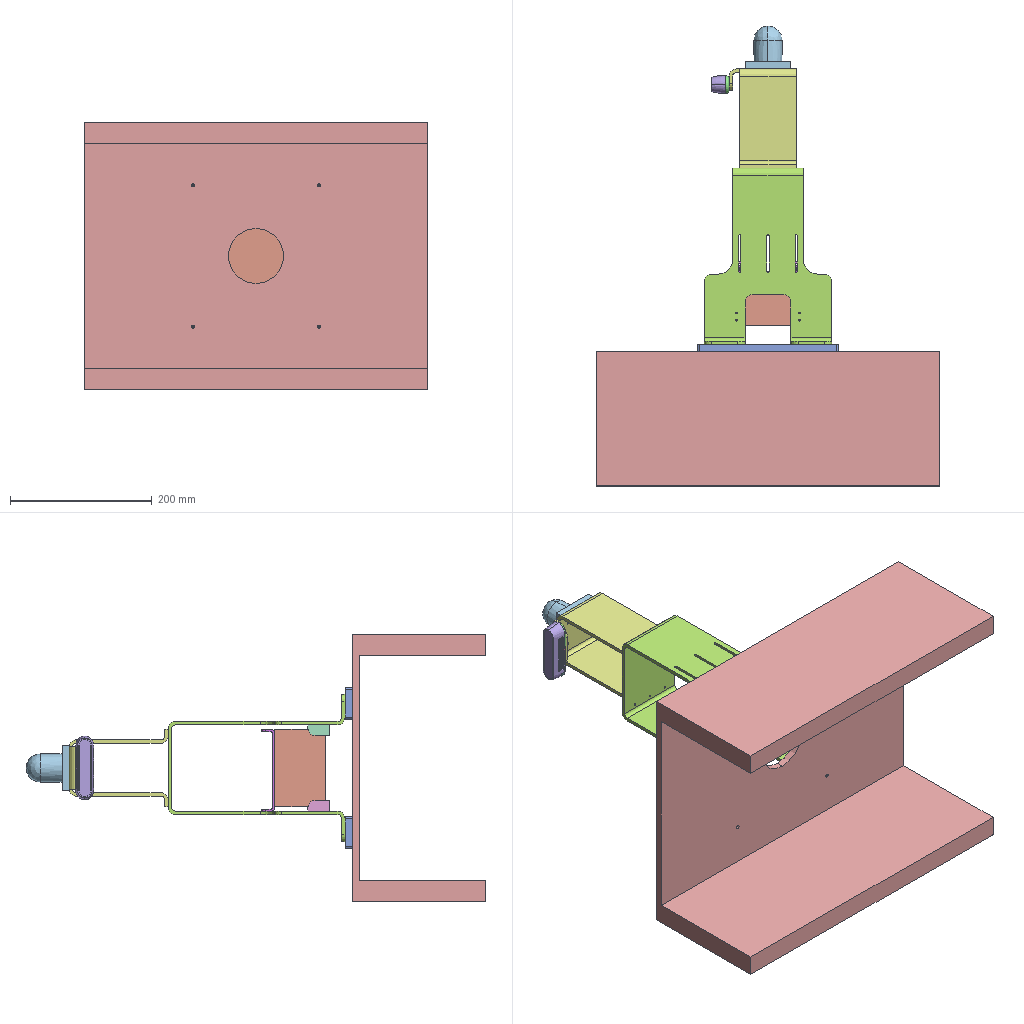Assembly | SolidWorks | 10 different items | 14 placed | box 484 x 650 x 378 mm
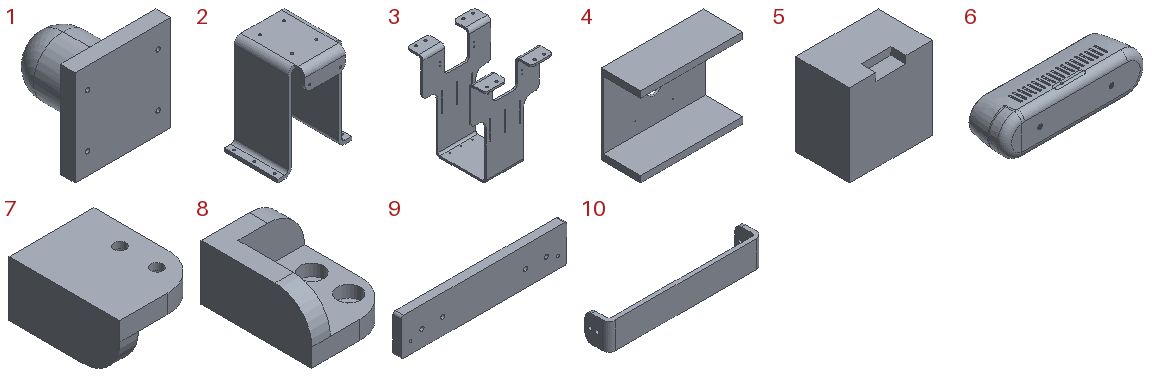Parts list (item | quantity | size | volume | features):
1 | x1 | 65 x 60.8 x 65 mm | 97568 mm3 | features ICE 2, Extrusion 1, Fillet 1
2 | x1 | 110 x 95 x 140 mm | 157187 mm3 | features ICE 7, Fillet 5, Extrusion 1
3 | x1 | 180 x 208 x 250 mm | 376013 mm3 | features ICE 8, Fillet 5, HoleWzd 2, MoveFace 2, Extrusion 1
4 | x1 | 484 x 189 x 378 mm | 6979121 mm3 | features ICE 2, Extrusion 1
5 | x1 | 110 x 72 x 110 mm | 863200 mm3 | features Extrusion 1, ICE 1
6 | x1 | 90 x 25 x 25 mm | 48696 mm3 | features ICE 13, SweepThread 3, Fillet 2, Split 2, Blend 1
7 | x2 | 23 x 30 x 15 mm | 5306 mm3 | features ICE 3, MoveFace 2, Extrusion 1, Fillet 1
8 | x2 | 23 x 30 x 15 mm | 5306 mm3 | features MirrorStock 1
9 | x2 | 200 x 10 x 45 mm | 88966 mm3 | features HoleWzd 2, MoveFace 2, Extrusion 1, Fillet 1
10 | x2 | 115 x 18 x 20 mm | 8396 mm3 | features Fillet 3, Extrusion 1, HoleWzd 1, ICE 1
Mates (type | each side: item.copy, entity, surface, feature):
Coincident | 4.1 face plane Boss-Extrude1 | 9.1 face plane Boss-Extrude1
Coincident | 4.1 face plane Boss-Extrude1 | 9.2 face plane Boss-Extrude1
Concentric | 4.1 face cylinder Cut-Extrude2 | 9.2 face cylinder M4 Tapped Hole1 | 2 times
Concentric | 4.1 face cylinder Cut-Extrude2 | 9.1 face cylinder M4 Tapped Hole1 | 2 times
Coincident | 9.1 face plane Boss-Extrude1 | 3.1 face plane Boss-Extrude3
Coincident | 3.1 face plane Boss-Extrude3 | 7.1 face plane Boss-Extrude1
Coincident | 3.1 face plane Boss-Extrude1 | 7.2 face plane Boss-Extrude1
Coincident | 3.1 face plane Boss-Extrude1 | 2.1 face plane Boss-Extrude1
DistanceDim | 2.1 face plane Boss-Extrude1 | 3.1 face plane Boss-Extrude1 | 2 times
Concentric | 9.2 face cylinder M6 Tapped Hole1 | 3.1 edge
Coincident | 6.1 face plane Boss-Extrude1 | 2.1 face plane Boss-Extrude4
Concentric | 6.1 select_type:24 | 2.1 face cylinder Cut-Extrude1 | 2 times
Coincident | 1.1 face plane Boss-Extrude1 | 2.1 face plane Boss-Extrude1
Concentric | 1.1 face cylinder Cut-Extrude1 | 2.1 face cylinder Cut-Extrude2 | 2 times
Coincident | 3.1 face plane Boss-Extrude1 | 10.1 face plane Boss-Extrude1
Parallel | 10.2 face plane Boss-Extrude1 | 10.1 face plane Boss-Extrude1
Coincident | 3.1 face plane Boss-Extrude1 | 10.2 face plane Boss-Extrude1
Coincident | 3.1 face plane Boss-Extrude3 | 8.1 face plane Angle IronMirror
Concentric | 3.1 face cylinder M3 Tapped Hole2 | 8.1 face cylinder Angle IronMirror | 2 times
Coincident | 3.1 face plane Boss-Extrude1 | 8.2 face plane Angle IronMirror
Concentric | 3.1 face cylinder M3 Tapped Hole2 | 8.2 face cylinder Angle IronMirror | 2 times
Coincident | 7.2 face plane Boss-Extrude2 | 5.1 face plane Boss-Extrude1
DistanceDim | 5.1 face plane Boss-Extrude1 | 7.2 face plane Boss-Extrude1
DistanceDim | 5.1 face plane Boss-Extrude1 | 8.1 face plane Angle IronMirror
Coincident | 10.2 face plane Boss-Extrude1 | 5.1 face plane Boss-Extrude1
Coincident | 10.1 face plane Boss-Extrude1 | 5.1 face plane Boss-Extrude1